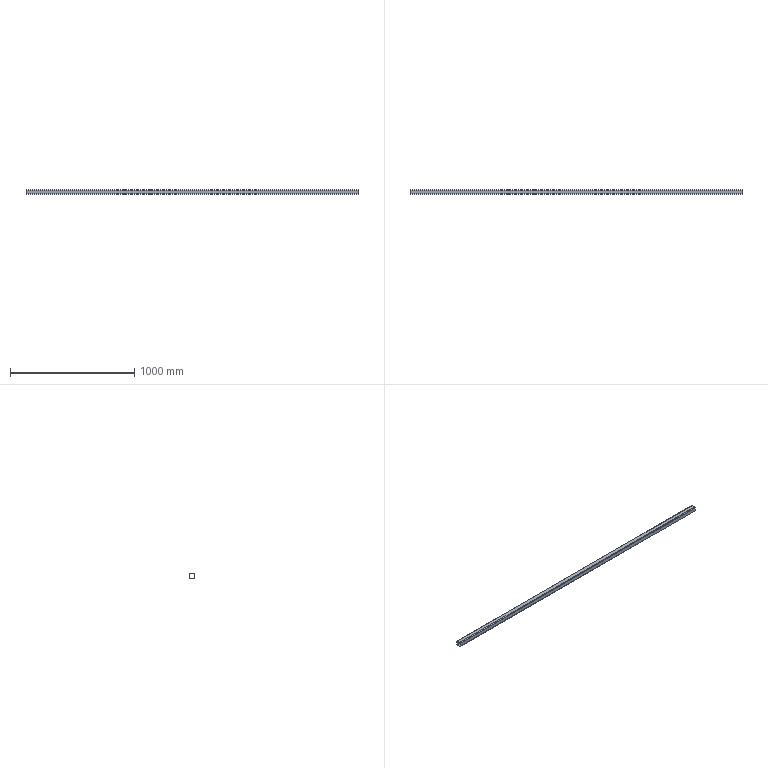Part | STEP file | VD-SYL0380DJ1006_1_2_1-5_STEP | 1 solid | 18 faces | box 2672 x 40 x 40 mm | volume 1124439 mm3 | plane 10 | cylinder 8 | commonest cylinder face diameters 6 x4 12 x4
STEP:
#1=CARTESIAN_POINT('',(1336.,-3.,-14.));
#2=VERTEX_POINT('',#1);
#3=CARTESIAN_POINT('',(1336.,-6.,-17.));
#4=VERTEX_POINT('',#3);
#5=CARTESIAN_POINT('',(1336.,-6.,-14.));
#6=DIRECTION('',(-1.,0.,0.));
#7=DIRECTION('',(0.,1.,0.));
#8=AXIS2_PLACEMENT_3D('',#5,#6,#7);
#9=CIRCLE('',#8,3.);
#10=EDGE_CURVE('',#2,#4,#9,.T.);
#11=ORIENTED_EDGE('',*,*,#10,.F.);
#12=CARTESIAN_POINT('',(-1336.,-3.,-14.));
#13=VERTEX_POINT('',#12);
#14=CARTESIAN_POINT('',(1336.,-3.,-14.));
#15=DIRECTION('',(-1.,0.,0.));
#16=VECTOR('',#15,1000.);
#17=LINE('',#14,#16);
#18=EDGE_CURVE('',#2,#13,#17,.T.);
#19=ORIENTED_EDGE('',*,*,#18,.T.);
#20=CARTESIAN_POINT('',(-1336.,-6.,-17.));
#21=VERTEX_POINT('',#20);
#22=CARTESIAN_POINT('',(-1336.,-6.,-14.));
#23=DIRECTION('',(1.,0.,0.));
#24=DIRECTION('',(0.,0.,-1.));
#25=AXIS2_PLACEMENT_3D('',#22,#23,#24);
#26=CIRCLE('',#25,3.);
#27=EDGE_CURVE('',#21,#13,#26,.T.);
#28=ORIENTED_EDGE('',*,*,#27,.F.);
#29=CARTESIAN_POINT('',(-1336.,-6.,-17.));
#30=DIRECTION('',(1.,0.,0.));
#31=VECTOR('',#30,1000.);
#32=LINE('',#29,#31);
#33=EDGE_CURVE('',#21,#4,#32,.T.);
#34=ORIENTED_EDGE('',*,*,#33,.T.);
#35=EDGE_LOOP('',(#11,#19,#28,#34));
#36=FACE_OUTER_BOUND('',#35,.T.);
#37=CARTESIAN_POINT('',(-1336.,-6.,-14.));
#38=DIRECTION('',(-1.,0.,0.));
#39=DIRECTION('',(0.,0.,1.));
#40=AXIS2_PLACEMENT_3D('',#37,#38,#39);
#41=CYLINDRICAL_SURFACE('',#40,3.);
#42=ADVANCED_FACE('',(#36),#41,.F.);
#43=CARTESIAN_POINT('',(-1336.,-3.,14.));
#44=VERTEX_POINT('',#43);
#45=CARTESIAN_POINT('',(1336.,-3.,14.));
#46=VERTEX_POINT('',#45);
#47=CARTESIAN_POINT('',(-1336.,-3.,14.));
#48=DIRECTION('',(1.,0.,0.));
#49=VECTOR('',#48,1000.);
#50=LINE('',#47,#49);
#51=EDGE_CURVE('',#44,#46,#50,.T.);
#52=ORIENTED_EDGE('',*,*,#51,.F.);
#53=CARTESIAN_POINT('',(-1336.,-3.,14.));
#54=DIRECTION('',(0.,0.,-1.));
#55=VECTOR('',#54,1000.);
#56=LINE('',#53,#55);
#57=EDGE_CURVE('',#44,#13,#56,.T.);
#58=ORIENTED_EDGE('',*,*,#57,.T.);
#59=ORIENTED_EDGE('',*,*,#18,.F.);
#60=CARTESIAN_POINT('',(1336.,-3.,14.));
#61=DIRECTION('',(0.,0.,-1.));
#62=VECTOR('',#61,1000.);
#63=LINE('',#60,#62);
#64=EDGE_CURVE('',#46,#2,#63,.T.);
#65=ORIENTED_EDGE('',*,*,#64,.F.);
#66=EDGE_LOOP('',(#52,#58,#59,#65));
#67=FACE_OUTER_BOUND('',#66,.T.);
#68=CARTESIAN_POINT('',(-1336.,-3.,-20.));
#69=DIRECTION('',(0.,1.,0.));
#70=DIRECTION('',(1.,0.,0.));
#71=AXIS2_PLACEMENT_3D('',#68,#69,#70);
#72=PLANE('',#71);
#73=ADVANCED_FACE('',(#67),#72,.F.);
#74=CARTESIAN_POINT('',(1336.,-6.,17.));
#75=VERTEX_POINT('',#74);
#76=CARTESIAN_POINT('',(1336.,-6.,14.));
#77=DIRECTION('',(-1.,0.,0.));
#78=DIRECTION('',(0.,0.,1.));
#79=AXIS2_PLACEMENT_3D('',#76,#77,#78);
#80=CIRCLE('',#79,3.);
#81=EDGE_CURVE('',#75,#46,#80,.T.);
#82=ORIENTED_EDGE('',*,*,#81,.F.);
#83=CARTESIAN_POINT('',(-1336.,-6.,17.));
#84=VERTEX_POINT('',#83);
#85=CARTESIAN_POINT('',(1336.,-6.,17.));
#86=DIRECTION('',(-1.,0.,0.));
#87=VECTOR('',#86,1000.);
#88=LINE('',#85,#87);
#89=EDGE_CURVE('',#75,#84,#88,.T.);
#90=ORIENTED_EDGE('',*,*,#89,.T.);
#91=CARTESIAN_POINT('',(-1336.,-6.,14.));
#92=DIRECTION('',(1.,0.,0.));
#93=DIRECTION('',(0.,1.,0.));
#94=AXIS2_PLACEMENT_3D('',#91,#92,#93);
#95=CIRCLE('',#94,3.);
#96=EDGE_CURVE('',#44,#84,#95,.T.);
#97=ORIENTED_EDGE('',*,*,#96,.F.);
#98=ORIENTED_EDGE('',*,*,#51,.T.);
#99=EDGE_LOOP('',(#82,#90,#97,#98));
#100=FACE_OUTER_BOUND('',#99,.T.);
#101=CARTESIAN_POINT('',(-1336.,-6.,14.));
#102=DIRECTION('',(-1.,0.,0.));
#103=DIRECTION('',(0.,0.,1.));
#104=AXIS2_PLACEMENT_3D('',#101,#102,#103);
#105=CYLINDRICAL_SURFACE('',#104,3.);
#106=ADVANCED_FACE('',(#100),#105,.F.);
#107=CARTESIAN_POINT('',(-1336.,-34.,17.));
#108=VERTEX_POINT('',#107);
#109=CARTESIAN_POINT('',(1336.,-34.,17.));
#110=VERTEX_POINT('',#109);
#111=CARTESIAN_POINT('',(-1336.,-34.,17.));
#112=DIRECTION('',(1.,0.,0.));
#113=VECTOR('',#112,1000.);
#114=LINE('',#111,#113);
#115=EDGE_CURVE('',#108,#110,#114,.T.);
#116=ORIENTED_EDGE('',*,*,#115,.F.);
#117=CARTESIAN_POINT('',(-1336.,-34.,17.));
#118=DIRECTION('',(0.,1.,0.));
#119=VECTOR('',#118,1000.);
#120=LINE('',#117,#119);
#121=EDGE_CURVE('',#108,#84,#120,.T.);
#122=ORIENTED_EDGE('',*,*,#121,.T.);
#123=ORIENTED_EDGE('',*,*,#89,.F.);
#124=CARTESIAN_POINT('',(1336.,-34.,17.));
#125=DIRECTION('',(0.,1.,0.));
#126=VECTOR('',#125,1000.);
#127=LINE('',#124,#126);
#128=EDGE_CURVE('',#110,#75,#127,.T.);
#129=ORIENTED_EDGE('',*,*,#128,.F.);
#130=EDGE_LOOP('',(#116,#122,#123,#129));
#131=FACE_OUTER_BOUND('',#130,.T.);
#132=CARTESIAN_POINT('',(-1336.,0.,17.));
#133=DIRECTION('',(0.,0.,1.));
#134=DIRECTION('',(1.,0.,0.));
#135=AXIS2_PLACEMENT_3D('',#132,#133,#134);
#136=PLANE('',#135);
#137=ADVANCED_FACE('',(#131),#136,.F.);
#138=CARTESIAN_POINT('',(1336.,-37.,14.));
#139=VERTEX_POINT('',#138);
#140=CARTESIAN_POINT('',(1336.,-34.,14.));
#141=DIRECTION('',(-1.,0.,0.));
#142=DIRECTION('',(0.,-1.,0.));
#143=AXIS2_PLACEMENT_3D('',#140,#141,#142);
#144=CIRCLE('',#143,3.);
#145=EDGE_CURVE('',#139,#110,#144,.T.);
#146=ORIENTED_EDGE('',*,*,#145,.F.);
#147=CARTESIAN_POINT('',(-1336.,-37.,14.));
#148=VERTEX_POINT('',#147);
#149=CARTESIAN_POINT('',(1336.,-37.,14.));
#150=DIRECTION('',(-1.,0.,0.));
#151=VECTOR('',#150,1000.);
#152=LINE('',#149,#151);
#153=EDGE_CURVE('',#139,#148,#152,.T.);
#154=ORIENTED_EDGE('',*,*,#153,.T.);
#155=CARTESIAN_POINT('',(-1336.,-34.,14.));
#156=DIRECTION('',(1.,0.,0.));
#157=DIRECTION('',(0.,0.,1.));
#158=AXIS2_PLACEMENT_3D('',#155,#156,#157);
#159=CIRCLE('',#158,3.);
#160=EDGE_CURVE('',#108,#148,#159,.T.);
#161=ORIENTED_EDGE('',*,*,#160,.F.);
#162=ORIENTED_EDGE('',*,*,#115,.T.);
#163=EDGE_LOOP('',(#146,#154,#161,#162));
#164=FACE_OUTER_BOUND('',#163,.T.);
#165=CARTESIAN_POINT('',(-1336.,-34.,14.));
#166=DIRECTION('',(-1.,0.,0.));
#167=DIRECTION('',(0.,0.,1.));
#168=AXIS2_PLACEMENT_3D('',#165,#166,#167);
#169=CYLINDRICAL_SURFACE('',#168,3.);
#170=ADVANCED_FACE('',(#164),#169,.F.);
#171=CARTESIAN_POINT('',(-1336.,-37.,-14.));
#172=VERTEX_POINT('',#171);
#173=CARTESIAN_POINT('',(1336.,-37.,-14.));
#174=VERTEX_POINT('',#173);
#175=CARTESIAN_POINT('',(-1336.,-37.,-14.));
#176=DIRECTION('',(1.,0.,0.));
#177=VECTOR('',#176,1000.);
#178=LINE('',#175,#177);
#179=EDGE_CURVE('',#172,#174,#178,.T.);
#180=ORIENTED_EDGE('',*,*,#179,.F.);
#181=CARTESIAN_POINT('',(-1336.,-37.,-14.));
#182=DIRECTION('',(0.,0.,1.));
#183=VECTOR('',#182,1000.);
#184=LINE('',#181,#183);
#185=EDGE_CURVE('',#172,#148,#184,.T.);
#186=ORIENTED_EDGE('',*,*,#185,.T.);
#187=ORIENTED_EDGE('',*,*,#153,.F.);
#188=CARTESIAN_POINT('',(1336.,-37.,-14.));
#189=DIRECTION('',(0.,0.,1.));
#190=VECTOR('',#189,1000.);
#191=LINE('',#188,#190);
#192=EDGE_CURVE('',#174,#139,#191,.T.);
#193=ORIENTED_EDGE('',*,*,#192,.F.);
#194=EDGE_LOOP('',(#180,#186,#187,#193));
#195=FACE_OUTER_BOUND('',#194,.T.);
#196=CARTESIAN_POINT('',(-1336.,-37.,20.));
#197=DIRECTION('',(0.,-1.,0.));
#198=DIRECTION('',(0.,0.,-1.));
#199=AXIS2_PLACEMENT_3D('',#196,#197,#198);
#200=PLANE('',#199);
#201=ADVANCED_FACE('',(#195),#200,.F.);
#202=CARTESIAN_POINT('',(1336.,-34.,-17.));
#203=VERTEX_POINT('',#202);
#204=CARTESIAN_POINT('',(1336.,-34.,-14.));
#205=DIRECTION('',(-1.,0.,0.));
#206=DIRECTION('',(0.,0.,-1.));
#207=AXIS2_PLACEMENT_3D('',#204,#205,#206);
#208=CIRCLE('',#207,3.);
#209=EDGE_CURVE('',#203,#174,#208,.T.);
#210=ORIENTED_EDGE('',*,*,#209,.F.);
#211=CARTESIAN_POINT('',(-1336.,-34.,-17.));
#212=VERTEX_POINT('',#211);
#213=CARTESIAN_POINT('',(1336.,-34.,-17.));
#214=DIRECTION('',(-1.,0.,0.));
#215=VECTOR('',#214,1000.);
#216=LINE('',#213,#215);
#217=EDGE_CURVE('',#203,#212,#216,.T.);
#218=ORIENTED_EDGE('',*,*,#217,.T.);
#219=CARTESIAN_POINT('',(-1336.,-34.,-14.));
#220=DIRECTION('',(1.,0.,0.));
#221=DIRECTION('',(0.,-1.,0.));
#222=AXIS2_PLACEMENT_3D('',#219,#220,#221);
#223=CIRCLE('',#222,3.);
#224=EDGE_CURVE('',#172,#212,#223,.T.);
#225=ORIENTED_EDGE('',*,*,#224,.F.);
#226=ORIENTED_EDGE('',*,*,#179,.T.);
#227=EDGE_LOOP('',(#210,#218,#225,#226));
#228=FACE_OUTER_BOUND('',#227,.T.);
#229=CARTESIAN_POINT('',(-1336.,-34.,-14.));
#230=DIRECTION('',(-1.,0.,0.));
#231=DIRECTION('',(0.,0.,1.));
#232=AXIS2_PLACEMENT_3D('',#229,#230,#231);
#233=CYLINDRICAL_SURFACE('',#232,3.);
#234=ADVANCED_FACE('',(#228),#233,.F.);
#235=ORIENTED_EDGE('',*,*,#33,.F.);
#236=CARTESIAN_POINT('',(-1336.,-6.,-17.));
#237=DIRECTION('',(0.,-1.,0.));
#238=VECTOR('',#237,1000.);
#239=LINE('',#236,#238);
#240=EDGE_CURVE('',#21,#212,#239,.T.);
#241=ORIENTED_EDGE('',*,*,#240,.T.);
#242=ORIENTED_EDGE('',*,*,#217,.F.);
#243=CARTESIAN_POINT('',(1336.,-6.,-17.));
#244=DIRECTION('',(0.,-1.,0.));
#245=VECTOR('',#244,1000.);
#246=LINE('',#243,#245);
#247=EDGE_CURVE('',#4,#203,#246,.T.);
#248=ORIENTED_EDGE('',*,*,#247,.F.);
#249=EDGE_LOOP('',(#235,#241,#242,#248));
#250=FACE_OUTER_BOUND('',#249,.T.);
#251=CARTESIAN_POINT('',(-1336.,-40.,-17.));
#252=DIRECTION('',(0.,0.,-1.));
#253=DIRECTION('',(0.,-1.,0.));
#254=AXIS2_PLACEMENT_3D('',#251,#252,#253);
#255=PLANE('',#254);
#256=ADVANCED_FACE('',(#250),#255,.F.);
#257=CARTESIAN_POINT('',(-1336.,0.,14.));
#258=VERTEX_POINT('',#257);
#259=CARTESIAN_POINT('',(-1336.,0.,-14.));
#260=VERTEX_POINT('',#259);
#261=CARTESIAN_POINT('',(-1336.,0.,14.));
#262=DIRECTION('',(0.,0.,-1.));
#263=VECTOR('',#262,1000.);
#264=LINE('',#261,#263);
#265=EDGE_CURVE('',#258,#260,#264,.T.);
#266=ORIENTED_EDGE('',*,*,#265,.F.);
#267=CARTESIAN_POINT('',(1336.,0.,14.));
#268=VERTEX_POINT('',#267);
#269=CARTESIAN_POINT('',(1336.,0.,14.));
#270=DIRECTION('',(-1.,0.,0.));
#271=VECTOR('',#270,1000.);
#272=LINE('',#269,#271);
#273=EDGE_CURVE('',#268,#258,#272,.T.);
#274=ORIENTED_EDGE('',*,*,#273,.F.);
#275=CARTESIAN_POINT('',(1336.,0.,-14.));
#276=VERTEX_POINT('',#275);
#277=CARTESIAN_POINT('',(1336.,0.,-14.));
#278=DIRECTION('',(0.,0.,1.));
#279=VECTOR('',#278,1000.);
#280=LINE('',#277,#279);
#281=EDGE_CURVE('',#276,#268,#280,.T.);
#282=ORIENTED_EDGE('',*,*,#281,.F.);
#283=CARTESIAN_POINT('',(-1336.,0.,-14.));
#284=DIRECTION('',(1.,0.,0.));
#285=VECTOR('',#284,1000.);
#286=LINE('',#283,#285);
#287=EDGE_CURVE('',#260,#276,#286,.T.);
#288=ORIENTED_EDGE('',*,*,#287,.F.);
#289=EDGE_LOOP('',(#266,#274,#282,#288));
#290=FACE_OUTER_BOUND('',#289,.T.);
#291=CARTESIAN_POINT('',(-1336.,0.,-20.));
#292=DIRECTION('',(0.,1.,0.));
#293=DIRECTION('',(1.,0.,0.));
#294=AXIS2_PLACEMENT_3D('',#291,#292,#293);
#295=PLANE('',#294);
#296=ADVANCED_FACE('',(#290),#295,.T.);
#297=ORIENTED_EDGE('',*,*,#209,.T.);
#298=ORIENTED_EDGE('',*,*,#192,.T.);
#299=ORIENTED_EDGE('',*,*,#145,.T.);
#300=ORIENTED_EDGE('',*,*,#128,.T.);
#301=ORIENTED_EDGE('',*,*,#81,.T.);
#302=ORIENTED_EDGE('',*,*,#64,.T.);
#303=ORIENTED_EDGE('',*,*,#10,.T.);
#304=ORIENTED_EDGE('',*,*,#247,.T.);
#305=EDGE_LOOP('',(#297,#298,#299,#300,#301,#302,#303,#304));
#306=FACE_BOUND('',#305,.T.);
#307=CARTESIAN_POINT('',(1336.,-34.,20.));
#308=VERTEX_POINT('',#307);
#309=CARTESIAN_POINT('',(1336.,-40.,14.));
#310=VERTEX_POINT('',#309);
#311=CARTESIAN_POINT('',(1336.,-34.,14.));
#312=DIRECTION('',(1.,0.,0.));
#313=DIRECTION('',(0.,0.,1.));
#314=AXIS2_PLACEMENT_3D('',#311,#312,#313);
#315=CIRCLE('',#314,6.);
#316=EDGE_CURVE('',#308,#310,#315,.T.);
#317=ORIENTED_EDGE('',*,*,#316,.T.);
#318=CARTESIAN_POINT('',(1336.,-40.,-14.));
#319=VERTEX_POINT('',#318);
#320=CARTESIAN_POINT('',(1336.,-40.,14.));
#321=DIRECTION('',(0.,0.,-1.));
#322=VECTOR('',#321,1000.);
#323=LINE('',#320,#322);
#324=EDGE_CURVE('',#310,#319,#323,.T.);
#325=ORIENTED_EDGE('',*,*,#324,.T.);
#326=CARTESIAN_POINT('',(1336.,-34.,-20.));
#327=VERTEX_POINT('',#326);
#328=CARTESIAN_POINT('',(1336.,-34.,-14.));
#329=DIRECTION('',(1.,0.,0.));
#330=DIRECTION('',(0.,-1.,0.));
#331=AXIS2_PLACEMENT_3D('',#328,#329,#330);
#332=CIRCLE('',#331,6.);
#333=EDGE_CURVE('',#319,#327,#332,.T.);
#334=ORIENTED_EDGE('',*,*,#333,.T.);
#335=CARTESIAN_POINT('',(1336.,-6.,-20.));
#336=VERTEX_POINT('',#335);
#337=CARTESIAN_POINT('',(1336.,-34.,-20.));
#338=DIRECTION('',(0.,1.,0.));
#339=VECTOR('',#338,1000.);
#340=LINE('',#337,#339);
#341=EDGE_CURVE('',#327,#336,#340,.T.);
#342=ORIENTED_EDGE('',*,*,#341,.T.);
#343=CARTESIAN_POINT('',(1336.,-6.,-14.));
#344=DIRECTION('',(1.,0.,0.));
#345=DIRECTION('',(0.,0.,-1.));
#346=AXIS2_PLACEMENT_3D('',#343,#344,#345);
#347=CIRCLE('',#346,6.);
#348=EDGE_CURVE('',#336,#276,#347,.T.);
#349=ORIENTED_EDGE('',*,*,#348,.T.);
#350=ORIENTED_EDGE('',*,*,#281,.T.);
#351=CARTESIAN_POINT('',(1336.,-6.,20.));
#352=VERTEX_POINT('',#351);
#353=CARTESIAN_POINT('',(1336.,-6.,14.));
#354=DIRECTION('',(1.,0.,0.));
#355=DIRECTION('',(0.,1.,0.));
#356=AXIS2_PLACEMENT_3D('',#353,#354,#355);
#357=CIRCLE('',#356,6.);
#358=EDGE_CURVE('',#268,#352,#357,.T.);
#359=ORIENTED_EDGE('',*,*,#358,.T.);
#360=CARTESIAN_POINT('',(1336.,-6.,20.));
#361=DIRECTION('',(0.,-1.,0.));
#362=VECTOR('',#361,1000.);
#363=LINE('',#360,#362);
#364=EDGE_CURVE('',#352,#308,#363,.T.);
#365=ORIENTED_EDGE('',*,*,#364,.T.);
#366=EDGE_LOOP('',(#317,#325,#334,#342,#349,#350,#359,#365));
#367=FACE_OUTER_BOUND('',#366,.T.);
#368=CARTESIAN_POINT('',(1336.,-20.,18.5));
#369=DIRECTION('',(-1.,0.,0.));
#370=DIRECTION('',(0.,0.,1.));
#371=AXIS2_PLACEMENT_3D('',#368,#369,#370);
#372=PLANE('',#371);
#373=ADVANCED_FACE('',(#306,#367),#372,.F.);
#374=CARTESIAN_POINT('',(-1336.,-40.,14.));
#375=VERTEX_POINT('',#374);
#376=CARTESIAN_POINT('',(-1336.,-40.,14.));
#377=DIRECTION('',(1.,0.,0.));
#378=VECTOR('',#377,1000.);
#379=LINE('',#376,#378);
#380=EDGE_CURVE('',#375,#310,#379,.T.);
#381=ORIENTED_EDGE('',*,*,#380,.T.);
#382=ORIENTED_EDGE('',*,*,#316,.F.);
#383=CARTESIAN_POINT('',(-1336.,-34.,20.));
#384=VERTEX_POINT('',#383);
#385=CARTESIAN_POINT('',(1336.,-34.,20.));
#386=DIRECTION('',(-1.,0.,0.));
#387=VECTOR('',#386,1000.);
#388=LINE('',#385,#387);
#389=EDGE_CURVE('',#308,#384,#388,.T.);
#390=ORIENTED_EDGE('',*,*,#389,.T.);
#391=CARTESIAN_POINT('',(-1336.,-34.,14.));
#392=DIRECTION('',(-1.,0.,0.));
#393=DIRECTION('',(0.,-1.,0.));
#394=AXIS2_PLACEMENT_3D('',#391,#392,#393);
#395=CIRCLE('',#394,6.);
#396=EDGE_CURVE('',#375,#384,#395,.T.);
#397=ORIENTED_EDGE('',*,*,#396,.F.);
#398=EDGE_LOOP('',(#381,#382,#390,#397));
#399=FACE_OUTER_BOUND('',#398,.T.);
#400=CARTESIAN_POINT('',(-1336.,-34.,14.));
#401=DIRECTION('',(-1.,0.,0.));
#402=DIRECTION('',(0.,0.,1.));
#403=AXIS2_PLACEMENT_3D('',#400,#401,#402);
#404=CYLINDRICAL_SURFACE('',#403,6.);
#405=ADVANCED_FACE('',(#399),#404,.T.);
#406=CARTESIAN_POINT('',(-1336.,-40.,-14.));
#407=VERTEX_POINT('',#406);
#408=CARTESIAN_POINT('',(-1336.,-40.,-14.));
#409=DIRECTION('',(0.,0.,1.));
#410=VECTOR('',#409,1000.);
#411=LINE('',#408,#410);
#412=EDGE_CURVE('',#407,#375,#411,.T.);
#413=ORIENTED_EDGE('',*,*,#412,.F.);
#414=CARTESIAN_POINT('',(1336.,-40.,-14.));
#415=DIRECTION('',(-1.,0.,0.));
#416=VECTOR('',#415,1000.);
#417=LINE('',#414,#416);
#418=EDGE_CURVE('',#319,#407,#417,.T.);
#419=ORIENTED_EDGE('',*,*,#418,.F.);
#420=ORIENTED_EDGE('',*,*,#324,.F.);
#421=ORIENTED_EDGE('',*,*,#380,.F.);
#422=EDGE_LOOP('',(#413,#419,#420,#421));
#423=FACE_OUTER_BOUND('',#422,.T.);
#424=CARTESIAN_POINT('',(-1336.,-40.,20.));
#425=DIRECTION('',(0.,-1.,0.));
#426=DIRECTION('',(0.,0.,-1.));
#427=AXIS2_PLACEMENT_3D('',#424,#425,#426);
#428=PLANE('',#427);
#429=ADVANCED_FACE('',(#423),#428,.T.);
#430=CARTESIAN_POINT('',(-1336.,-34.,-20.));
#431=VERTEX_POINT('',#430);
#432=CARTESIAN_POINT('',(-1336.,-34.,-20.));
#433=DIRECTION('',(1.,0.,0.));
#434=VECTOR('',#433,1000.);
#435=LINE('',#432,#434);
#436=EDGE_CURVE('',#431,#327,#435,.T.);
#437=ORIENTED_EDGE('',*,*,#436,.T.);
#438=ORIENTED_EDGE('',*,*,#333,.F.);
#439=ORIENTED_EDGE('',*,*,#418,.T.);
#440=CARTESIAN_POINT('',(-1336.,-34.,-14.));
#441=DIRECTION('',(-1.,0.,0.));
#442=DIRECTION('',(0.,0.,-1.));
#443=AXIS2_PLACEMENT_3D('',#440,#441,#442);
#444=CIRCLE('',#443,6.);
#445=EDGE_CURVE('',#431,#407,#444,.T.);
#446=ORIENTED_EDGE('',*,*,#445,.F.);
#447=EDGE_LOOP('',(#437,#438,#439,#446));
#448=FACE_OUTER_BOUND('',#447,.T.);
#449=CARTESIAN_POINT('',(-1336.,-34.,-14.));
#450=DIRECTION('',(-1.,0.,0.));
#451=DIRECTION('',(0.,0.,1.));
#452=AXIS2_PLACEMENT_3D('',#449,#450,#451);
#453=CYLINDRICAL_SURFACE('',#452,6.);
#454=ADVANCED_FACE('',(#448),#453,.T.);
#455=CARTESIAN_POINT('',(-1336.,-6.,-20.));
#456=VERTEX_POINT('',#455);
#457=CARTESIAN_POINT('',(-1336.,-6.,-20.));
#458=DIRECTION('',(0.,-1.,0.));
#459=VECTOR('',#458,1000.);
#460=LINE('',#457,#459);
#461=EDGE_CURVE('',#456,#431,#460,.T.);
#462=ORIENTED_EDGE('',*,*,#461,.F.);
#463=CARTESIAN_POINT('',(1336.,-6.,-20.));
#464=DIRECTION('',(-1.,0.,0.));
#465=VECTOR('',#464,1000.);
#466=LINE('',#463,#465);
#467=EDGE_CURVE('',#336,#456,#466,.T.);
#468=ORIENTED_EDGE('',*,*,#467,.F.);
#469=ORIENTED_EDGE('',*,*,#341,.F.);
#470=ORIENTED_EDGE('',*,*,#436,.F.);
#471=EDGE_LOOP('',(#462,#468,#469,#470));
#472=FACE_OUTER_BOUND('',#471,.T.);
#473=CARTESIAN_POINT('',(-1336.,-40.,-20.));
#474=DIRECTION('',(0.,0.,-1.));
#475=DIRECTION('',(0.,-1.,0.));
#476=AXIS2_PLACEMENT_3D('',#473,#474,#475);
#477=PLANE('',#476);
#478=ADVANCED_FACE('',(#472),#477,.T.);
#479=ORIENTED_EDGE('',*,*,#287,.T.);
#480=ORIENTED_EDGE('',*,*,#348,.F.);
#481=ORIENTED_EDGE('',*,*,#467,.T.);
#482=CARTESIAN_POINT('',(-1336.,-6.,-14.));
#483=DIRECTION('',(-1.,0.,0.));
#484=DIRECTION('',(0.,1.,0.));
#485=AXIS2_PLACEMENT_3D('',#482,#483,#484);
#486=CIRCLE('',#485,6.);
#487=EDGE_CURVE('',#260,#456,#486,.T.);
#488=ORIENTED_EDGE('',*,*,#487,.F.);
#489=EDGE_LOOP('',(#479,#480,#481,#488));
#490=FACE_OUTER_BOUND('',#489,.T.);
#491=CARTESIAN_POINT('',(-1336.,-6.,-14.));
#492=DIRECTION('',(-1.,0.,0.));
#493=DIRECTION('',(0.,0.,1.));
#494=AXIS2_PLACEMENT_3D('',#491,#492,#493);
#495=CYLINDRICAL_SURFACE('',#494,6.);
#496=ADVANCED_FACE('',(#490),#495,.T.);
#497=ORIENTED_EDGE('',*,*,#160,.T.);
#498=ORIENTED_EDGE('',*,*,#185,.F.);
#499=ORIENTED_EDGE('',*,*,#224,.T.);
#500=ORIENTED_EDGE('',*,*,#240,.F.);
#501=ORIENTED_EDGE('',*,*,#27,.T.);
#502=ORIENTED_EDGE('',*,*,#57,.F.);
#503=ORIENTED_EDGE('',*,*,#96,.T.);
#504=ORIENTED_EDGE('',*,*,#121,.F.);
#505=EDGE_LOOP('',(#497,#498,#499,#500,#501,#502,#503,#504));
#506=FACE_BOUND('',#505,.T.);
#507=ORIENTED_EDGE('',*,*,#461,.T.);
#508=ORIENTED_EDGE('',*,*,#445,.T.);
#509=ORIENTED_EDGE('',*,*,#412,.T.);
#510=ORIENTED_EDGE('',*,*,#396,.T.);
#511=CARTESIAN_POINT('',(-1336.,-6.,20.));
#512=VERTEX_POINT('',#511);
#513=CARTESIAN_POINT('',(-1336.,-34.,20.));
#514=DIRECTION('',(0.,1.,0.));
#515=VECTOR('',#514,1000.);
#516=LINE('',#513,#515);
#517=EDGE_CURVE('',#384,#512,#516,.T.);
#518=ORIENTED_EDGE('',*,*,#517,.T.);
#519=CARTESIAN_POINT('',(-1336.,-6.,14.));
#520=DIRECTION('',(-1.,0.,0.));
#521=DIRECTION('',(0.,0.,1.));
#522=AXIS2_PLACEMENT_3D('',#519,#520,#521);
#523=CIRCLE('',#522,6.);
#524=EDGE_CURVE('',#512,#258,#523,.T.);
#525=ORIENTED_EDGE('',*,*,#524,.T.);
#526=ORIENTED_EDGE('',*,*,#265,.T.);
#527=ORIENTED_EDGE('',*,*,#487,.T.);
#528=EDGE_LOOP('',(#507,#508,#509,#510,#518,#525,#526,#527));
#529=FACE_OUTER_BOUND('',#528,.T.);
#530=CARTESIAN_POINT('',(-1336.,-20.,18.5));
#531=DIRECTION('',(-1.,0.,0.));
#532=DIRECTION('',(0.,0.,1.));
#533=AXIS2_PLACEMENT_3D('',#530,#531,#532);
#534=PLANE('',#533);
#535=ADVANCED_FACE('',(#506,#529),#534,.T.);
#536=CARTESIAN_POINT('',(-1336.,-6.,20.));
#537=DIRECTION('',(1.,0.,0.));
#538=VECTOR('',#537,1000.);
#539=LINE('',#536,#538);
#540=EDGE_CURVE('',#512,#352,#539,.T.);
#541=ORIENTED_EDGE('',*,*,#540,.T.);
#542=ORIENTED_EDGE('',*,*,#358,.F.);
#543=ORIENTED_EDGE('',*,*,#273,.T.);
#544=ORIENTED_EDGE('',*,*,#524,.F.);
#545=EDGE_LOOP('',(#541,#542,#543,#544));
#546=FACE_OUTER_BOUND('',#545,.T.);
#547=CARTESIAN_POINT('',(-1336.,-6.,14.));
#548=DIRECTION('',(-1.,0.,0.));
#549=DIRECTION('',(0.,0.,1.));
#550=AXIS2_PLACEMENT_3D('',#547,#548,#549);
#551=CYLINDRICAL_SURFACE('',#550,6.);
#552=ADVANCED_FACE('',(#546),#551,.T.);
#553=ORIENTED_EDGE('',*,*,#517,.F.);
#554=ORIENTED_EDGE('',*,*,#389,.F.);
#555=ORIENTED_EDGE('',*,*,#364,.F.);
#556=ORIENTED_EDGE('',*,*,#540,.F.);
#557=EDGE_LOOP('',(#553,#554,#555,#556));
#558=FACE_OUTER_BOUND('',#557,.T.);
#559=CARTESIAN_POINT('',(-1336.,0.,20.));
#560=DIRECTION('',(0.,0.,1.));
#561=DIRECTION('',(1.,0.,0.));
#562=AXIS2_PLACEMENT_3D('',#559,#560,#561);
#563=PLANE('',#562);
#564=ADVANCED_FACE('',(#558),#563,.T.);
#565=CLOSED_SHELL('',(#42,#73,#106,#137,#170,#201,#234,#256,#296,#373,#405,#429,#454,#478,#496,#535,#552,#564));
#566=MANIFOLD_SOLID_BREP('',#565);
#567=CARTESIAN_POINT('',(0.,0.,0.));
#568=DIRECTION('',(0.,0.,1.));
#569=DIRECTION('',(1.,0.,0.));
#570=AXIS2_PLACEMENT_3D('',#567,#568,#569);
#571=(LENGTH_UNIT()NAMED_UNIT(*)SI_UNIT(.MILLI.,.METRE.));
#572=UNCERTAINTY_MEASURE_WITH_UNIT(LENGTH_MEASURE(0.00001),#571,'','');
#573=(NAMED_UNIT(*)PLANE_ANGLE_UNIT()SI_UNIT($,.RADIAN.));
#574=(NAMED_UNIT(*)SI_UNIT($,.STERADIAN.)SOLID_ANGLE_UNIT());
#575=(GEOMETRIC_REPRESENTATION_CONTEXT(3)GLOBAL_UNCERTAINTY_ASSIGNED_CONTEXT((#572))GLOBAL_UNIT_ASSIGNED_CONTEXT((#571,#573,#574))REPRESENTATION_CONTEXT('',''));
#576=ADVANCED_BREP_SHAPE_REPRESENTATION('',(#566,#570),#575);